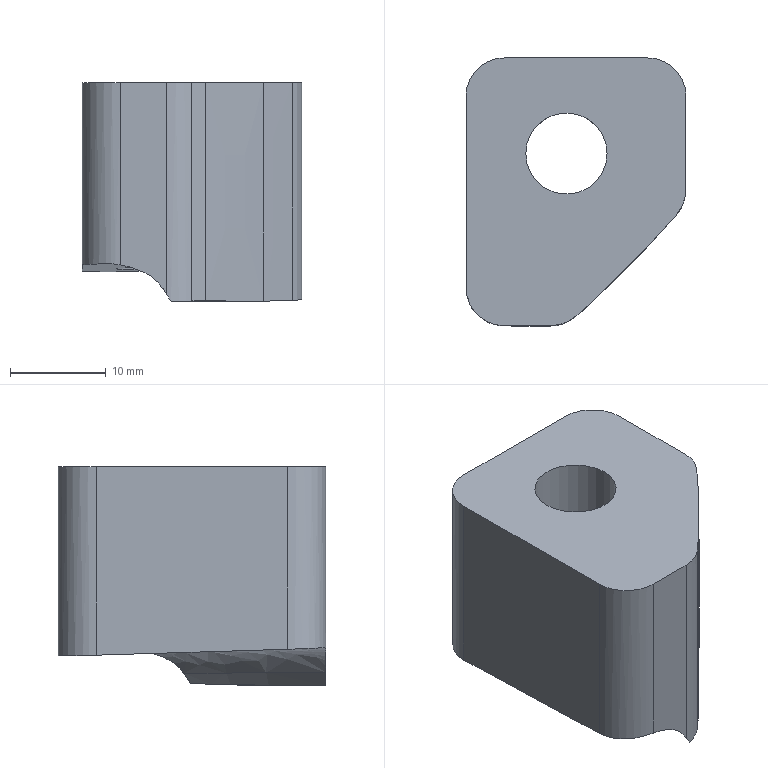Part | STEP file | gslz 2016.10.28-10_id1230_x_t | 1 solid | 21 faces | box 23 x 28 x 22.89 mm | volume 8664 mm3 | cylinder 7 | plane 6 | spline 5 | other 3 | commonest cylinder face diameters 8 x5 8.5 x1 14 x1